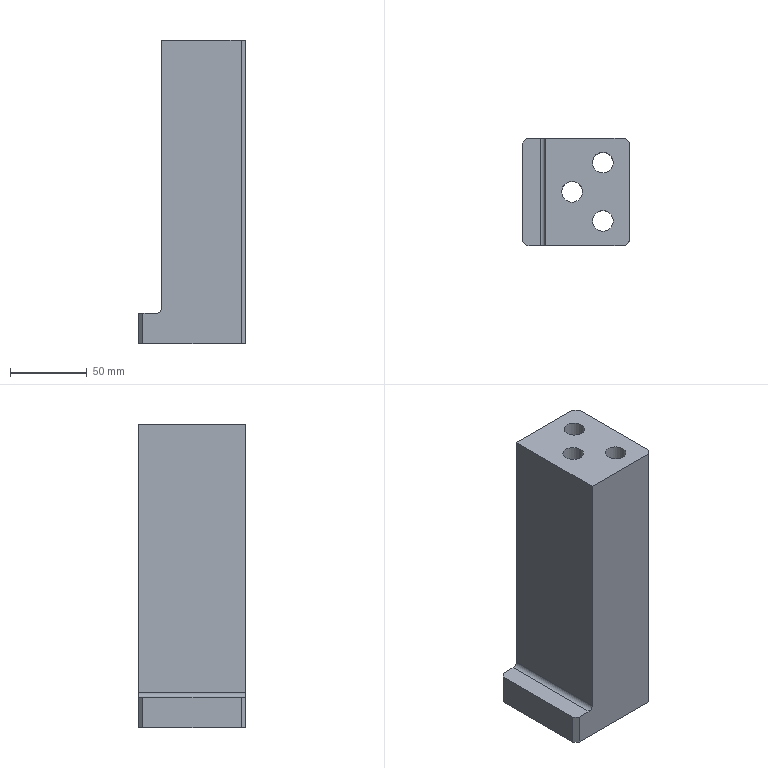Part | NX | features solid 2 | 1 solid | 22 faces | box 70 x 70 x 198 mm | volume 634687 mm3 | plane 15 | cylinder 7 | commonest cylinder face diameters 13.507 x3 20.008 x3 6 x1
STEP:
#1=CARTESIAN_POINT('',(964.467,186.199,-16.87));
#2=VERTEX_POINT('',#1);
#3=CARTESIAN_POINT('',(964.467,122.199,-16.87));
#4=VERTEX_POINT('',#3);
#5=CARTESIAN_POINT('',(964.467,12.095,-16.87));
#6=DIRECTION('',(0.,-1.,0.));
#7=VECTOR('',#6,1000.);
#8=LINE('',#5,#7);
#9=EDGE_CURVE('',#2,#4,#8,.T.);
#10=ORIENTED_EDGE('',*,*,#9,.T.);
#11=CARTESIAN_POINT('',(961.467,119.199,-16.87));
#12=VERTEX_POINT('',#11);
#13=CARTESIAN_POINT('',(777.169,-65.098,-16.87));
#14=DIRECTION('',(0.7071,0.7071,0.));
#15=VECTOR('',#14,1000.);
#16=LINE('',#13,#15);
#17=EDGE_CURVE('',#4,#12,#16,.F.);
#18=ORIENTED_EDGE('',*,*,#17,.T.);
#19=CARTESIAN_POINT('',(897.467,119.199,-16.87));
#20=VERTEX_POINT('',#19);
#21=CARTESIAN_POINT('',(699.976,119.199,-16.87));
#22=DIRECTION('',(-1.,0.,0.));
#23=VECTOR('',#22,1000.);
#24=LINE('',#21,#23);
#25=EDGE_CURVE('',#12,#20,#24,.T.);
#26=ORIENTED_EDGE('',*,*,#25,.T.);
#27=CARTESIAN_POINT('',(894.467,122.199,-16.87));
#28=VERTEX_POINT('',#27);
#29=CARTESIAN_POINT('',(852.274,164.392,-16.87));
#30=DIRECTION('',(0.7071,-0.7071,0.));
#31=VECTOR('',#30,1000.);
#32=LINE('',#29,#31);
#33=EDGE_CURVE('',#20,#28,#32,.F.);
#34=ORIENTED_EDGE('',*,*,#33,.T.);
#35=CARTESIAN_POINT('',(894.467,186.199,-16.87));
#36=VERTEX_POINT('',#35);
#37=CARTESIAN_POINT('',(894.467,12.095,-16.87));
#38=DIRECTION('',(0.,1.,0.));
#39=VECTOR('',#38,1000.);
#40=LINE('',#37,#39);
#41=EDGE_CURVE('',#28,#36,#40,.T.);
#42=ORIENTED_EDGE('',*,*,#41,.T.);
#43=CARTESIAN_POINT('',(897.467,189.199,-16.87));
#44=VERTEX_POINT('',#43);
#45=CARTESIAN_POINT('',(710.169,1.902,-16.87));
#46=DIRECTION('',(-0.7071,-0.7071,0.));
#47=VECTOR('',#46,1000.);
#48=LINE('',#45,#47);
#49=EDGE_CURVE('',#36,#44,#48,.F.);
#50=ORIENTED_EDGE('',*,*,#49,.T.);
#51=CARTESIAN_POINT('',(961.467,189.199,-16.87));
#52=VERTEX_POINT('',#51);
#53=CARTESIAN_POINT('',(699.976,189.199,-16.87));
#54=DIRECTION('',(1.,0.,0.));
#55=VECTOR('',#54,1000.);
#56=LINE('',#53,#55);
#57=EDGE_CURVE('',#44,#52,#56,.T.);
#58=ORIENTED_EDGE('',*,*,#57,.T.);
#59=CARTESIAN_POINT('',(919.274,231.392,-16.87));
#60=DIRECTION('',(-0.7071,0.7071,0.));
#61=VECTOR('',#60,1000.);
#62=LINE('',#59,#61);
#63=EDGE_CURVE('',#52,#2,#62,.F.);
#64=ORIENTED_EDGE('',*,*,#63,.T.);
#65=EDGE_LOOP('',(#10,#18,#26,#34,#42,#50,#58,#64));
#66=FACE_BOUND('',#65,.T.);
#67=CARTESIAN_POINT('',(936.963,135.199,-16.87));
#68=VERTEX_POINT('',#67);
#69=CARTESIAN_POINT('',(946.967,135.199,-16.87));
#70=DIRECTION('',(0.,0.,-1.));
#71=DIRECTION('',(-1.,0.,0.));
#72=AXIS2_PLACEMENT_3D('',#69,#70,#71);
#73=CIRCLE('',#72,10.004);
#74=EDGE_CURVE('',#68,#68,#73,.T.);
#75=ORIENTED_EDGE('',*,*,#74,.F.);
#76=EDGE_LOOP('',(#75));
#77=FACE_BOUND('',#76,.T.);
#78=CARTESIAN_POINT('',(936.963,173.199,-16.87));
#79=VERTEX_POINT('',#78);
#80=CARTESIAN_POINT('',(946.967,173.199,-16.87));
#81=DIRECTION('',(0.,0.,-1.));
#82=DIRECTION('',(-1.,0.,0.));
#83=AXIS2_PLACEMENT_3D('',#80,#81,#82);
#84=CIRCLE('',#83,10.004);
#85=EDGE_CURVE('',#79,#79,#84,.T.);
#86=ORIENTED_EDGE('',*,*,#85,.F.);
#87=EDGE_LOOP('',(#86));
#88=FACE_BOUND('',#87,.T.);
#89=CARTESIAN_POINT('',(916.963,154.199,-16.87));
#90=VERTEX_POINT('',#89);
#91=CARTESIAN_POINT('',(926.967,154.199,-16.87));
#92=DIRECTION('',(0.,0.,-1.));
#93=DIRECTION('',(-1.,0.,0.));
#94=AXIS2_PLACEMENT_3D('',#91,#92,#93);
#95=CIRCLE('',#94,10.004);
#96=EDGE_CURVE('',#90,#90,#95,.F.);
#97=ORIENTED_EDGE('',*,*,#96,.T.);
#98=EDGE_LOOP('',(#97));
#99=FACE_BOUND('',#98,.T.);
#100=CARTESIAN_POINT('',(699.976,12.095,-16.87));
#101=DIRECTION('',(0.,0.,-1.));
#102=DIRECTION('',(-1.,0.,0.));
#103=AXIS2_PLACEMENT_3D('',#100,#101,#102);
#104=PLANE('',#103);
#105=ADVANCED_FACE('',(#66,#77,#88,#99),#104,.T.);
#106=CARTESIAN_POINT('',(894.467,186.199,2.999));
#107=VERTEX_POINT('',#106);
#108=CARTESIAN_POINT('',(894.467,122.199,2.999));
#109=VERTEX_POINT('',#108);
#110=CARTESIAN_POINT('',(894.467,189.199,2.999));
#111=DIRECTION('',(0.,1.,0.));
#112=VECTOR('',#111,1000.);
#113=LINE('',#110,#112);
#114=EDGE_CURVE('',#107,#109,#113,.F.);
#115=ORIENTED_EDGE('',*,*,#114,.T.);
#116=CARTESIAN_POINT('',(897.467,119.199,2.999));
#117=VERTEX_POINT('',#116);
#118=CARTESIAN_POINT('',(894.467,122.199,2.999));
#119=DIRECTION('',(0.7071,-0.7071,0.));
#120=VECTOR('',#119,1000.);
#121=LINE('',#118,#120);
#122=EDGE_CURVE('',#109,#117,#121,.T.);
#123=ORIENTED_EDGE('',*,*,#122,.T.);
#124=CARTESIAN_POINT('',(906.467,119.199,2.999));
#125=VERTEX_POINT('',#124);
#126=CARTESIAN_POINT('',(894.467,119.199,2.999));
#127=DIRECTION('',(-1.,0.,0.));
#128=VECTOR('',#127,1000.);
#129=LINE('',#126,#128);
#130=EDGE_CURVE('',#117,#125,#129,.F.);
#131=ORIENTED_EDGE('',*,*,#130,.T.);
#132=CARTESIAN_POINT('',(906.467,189.199,2.999));
#133=VERTEX_POINT('',#132);
#134=CARTESIAN_POINT('',(906.467,154.199,2.999));
#135=DIRECTION('',(0.,1.,0.));
#136=VECTOR('',#135,1000.);
#137=LINE('',#134,#136);
#138=EDGE_CURVE('',#125,#133,#137,.T.);
#139=ORIENTED_EDGE('',*,*,#138,.T.);
#140=CARTESIAN_POINT('',(897.467,189.199,2.999));
#141=VERTEX_POINT('',#140);
#142=CARTESIAN_POINT('',(959.467,189.199,2.999));
#143=DIRECTION('',(1.,0.,0.));
#144=VECTOR('',#143,1000.);
#145=LINE('',#142,#144);
#146=EDGE_CURVE('',#133,#141,#145,.F.);
#147=ORIENTED_EDGE('',*,*,#146,.T.);
#148=CARTESIAN_POINT('',(897.467,189.199,2.999));
#149=DIRECTION('',(-0.7071,-0.7071,0.));
#150=VECTOR('',#149,1000.);
#151=LINE('',#148,#150);
#152=EDGE_CURVE('',#141,#107,#151,.T.);
#153=ORIENTED_EDGE('',*,*,#152,.T.);
#154=EDGE_LOOP('',(#115,#123,#131,#139,#147,#153));
#155=FACE_BOUND('',#154,.T.);
#156=CARTESIAN_POINT('',(926.967,154.199,2.999));
#157=DIRECTION('',(0.,0.,-1.));
#158=DIRECTION('',(0.,-1.,0.));
#159=AXIS2_PLACEMENT_3D('',#156,#157,#158);
#160=PLANE('',#159);
#161=ADVANCED_FACE('',(#155),#160,.F.);
#162=CARTESIAN_POINT('',(909.467,119.199,5.999));
#163=VERTEX_POINT('',#162);
#164=CARTESIAN_POINT('',(906.467,119.199,5.999));
#165=DIRECTION('',(0.,1.,0.));
#166=DIRECTION('',(0.,0.,1.));
#167=AXIS2_PLACEMENT_3D('',#164,#165,#166);
#168=CIRCLE('',#167,3.);
#169=EDGE_CURVE('',#163,#125,#168,.T.);
#170=ORIENTED_EDGE('',*,*,#169,.F.);
#171=CARTESIAN_POINT('',(909.467,189.199,5.999));
#172=VERTEX_POINT('',#171);
#173=CARTESIAN_POINT('',(909.467,189.199,5.999));
#174=DIRECTION('',(0.,1.,0.));
#175=VECTOR('',#174,1000.);
#176=LINE('',#173,#175);
#177=EDGE_CURVE('',#172,#163,#176,.F.);
#178=ORIENTED_EDGE('',*,*,#177,.F.);
#179=CARTESIAN_POINT('',(906.467,189.199,5.999));
#180=DIRECTION('',(0.,-1.,0.));
#181=DIRECTION('',(0.,0.,-1.));
#182=AXIS2_PLACEMENT_3D('',#179,#180,#181);
#183=CIRCLE('',#182,3.);
#184=EDGE_CURVE('',#133,#172,#183,.T.);
#185=ORIENTED_EDGE('',*,*,#184,.F.);
#186=ORIENTED_EDGE('',*,*,#138,.F.);
#187=EDGE_LOOP('',(#170,#178,#185,#186));
#188=FACE_BOUND('',#187,.T.);
#189=CARTESIAN_POINT('',(906.467,189.199,5.999));
#190=DIRECTION('',(0.,1.,0.));
#191=DIRECTION('',(0.,0.,-1.));
#192=AXIS2_PLACEMENT_3D('',#189,#190,#191);
#193=CYLINDRICAL_SURFACE('',#192,3.);
#194=ADVANCED_FACE('',(#188),#193,.F.);
#195=CARTESIAN_POINT('',(909.467,119.199,181.13));
#196=VERTEX_POINT('',#195);
#197=CARTESIAN_POINT('',(909.467,119.199,194.799));
#198=DIRECTION('',(0.,0.,-1.));
#199=VECTOR('',#198,1000.);
#200=LINE('',#197,#199);
#201=EDGE_CURVE('',#163,#196,#200,.F.);
#202=ORIENTED_EDGE('',*,*,#201,.T.);
#203=CARTESIAN_POINT('',(909.467,189.199,181.13));
#204=VERTEX_POINT('',#203);
#205=CARTESIAN_POINT('',(909.467,-371.311,181.13));
#206=DIRECTION('',(0.,1.,0.));
#207=VECTOR('',#206,1000.);
#208=LINE('',#205,#207);
#209=EDGE_CURVE('',#196,#204,#208,.T.);
#210=ORIENTED_EDGE('',*,*,#209,.T.);
#211=CARTESIAN_POINT('',(909.467,189.199,194.799));
#212=DIRECTION('',(0.,0.,-1.));
#213=VECTOR('',#212,1000.);
#214=LINE('',#211,#213);
#215=EDGE_CURVE('',#172,#204,#214,.F.);
#216=ORIENTED_EDGE('',*,*,#215,.F.);
#217=ORIENTED_EDGE('',*,*,#177,.T.);
#218=EDGE_LOOP('',(#202,#210,#216,#217));
#219=FACE_BOUND('',#218,.T.);
#220=CARTESIAN_POINT('',(909.467,189.199,194.799));
#221=DIRECTION('',(-1.,0.,0.));
#222=DIRECTION('',(0.,0.,-1.));
#223=AXIS2_PLACEMENT_3D('',#220,#221,#222);
#224=PLANE('',#223);
#225=ADVANCED_FACE('',(#219),#224,.T.);
#226=CARTESIAN_POINT('',(961.467,119.199,181.13));
#227=VERTEX_POINT('',#226);
#228=CARTESIAN_POINT('',(964.467,122.199,181.13));
#229=VERTEX_POINT('',#228);
#230=CARTESIAN_POINT('',(961.467,119.199,181.13));
#231=DIRECTION('',(-0.7071,-0.7071,0.));
#232=VECTOR('',#231,1000.);
#233=LINE('',#230,#232);
#234=EDGE_CURVE('',#227,#229,#233,.F.);
#235=ORIENTED_EDGE('',*,*,#234,.F.);
#236=CARTESIAN_POINT('',(961.467,119.199,194.799));
#237=DIRECTION('',(0.,0.,-1.));
#238=VECTOR('',#237,1000.);
#239=LINE('',#236,#238);
#240=EDGE_CURVE('',#12,#227,#239,.F.);
#241=ORIENTED_EDGE('',*,*,#240,.F.);
#242=ORIENTED_EDGE('',*,*,#17,.F.);
#243=CARTESIAN_POINT('',(964.467,122.199,194.799));
#244=DIRECTION('',(0.,0.,1.));
#245=VECTOR('',#244,1000.);
#246=LINE('',#243,#245);
#247=EDGE_CURVE('',#229,#4,#246,.F.);
#248=ORIENTED_EDGE('',*,*,#247,.F.);
#249=EDGE_LOOP('',(#235,#241,#242,#248));
#250=FACE_BOUND('',#249,.T.);
#251=CARTESIAN_POINT('',(961.467,119.199,194.799));
#252=DIRECTION('',(-0.7071,0.7071,0.));
#253=DIRECTION('',(0.7071,0.7071,0.));
#254=AXIS2_PLACEMENT_3D('',#251,#252,#253);
#255=PLANE('',#254);
#256=ADVANCED_FACE('',(#250),#255,.F.);
#257=CARTESIAN_POINT('',(729.857,119.199,181.13));
#258=DIRECTION('',(-1.,0.,0.));
#259=VECTOR('',#258,1000.);
#260=LINE('',#257,#259);
#261=EDGE_CURVE('',#227,#196,#260,.T.);
#262=ORIENTED_EDGE('',*,*,#261,.T.);
#263=ORIENTED_EDGE('',*,*,#201,.F.);
#264=ORIENTED_EDGE('',*,*,#169,.T.);
#265=ORIENTED_EDGE('',*,*,#130,.F.);
#266=CARTESIAN_POINT('',(897.467,119.199,122.999));
#267=DIRECTION('',(0.,0.,1.));
#268=VECTOR('',#267,1000.);
#269=LINE('',#266,#268);
#270=EDGE_CURVE('',#117,#20,#269,.F.);
#271=ORIENTED_EDGE('',*,*,#270,.T.);
#272=ORIENTED_EDGE('',*,*,#25,.F.);
#273=ORIENTED_EDGE('',*,*,#240,.T.);
#274=EDGE_LOOP('',(#262,#263,#264,#265,#271,#272,#273));
#275=FACE_BOUND('',#274,.T.);
#276=CARTESIAN_POINT('',(894.467,119.199,194.799));
#277=DIRECTION('',(0.,-1.,0.));
#278=DIRECTION('',(0.,0.,1.));
#279=AXIS2_PLACEMENT_3D('',#276,#277,#278);
#280=PLANE('',#279);
#281=ADVANCED_FACE('',(#275),#280,.T.);
#282=ORIENTED_EDGE('',*,*,#122,.F.);
#283=CARTESIAN_POINT('',(894.467,122.199,122.999));
#284=DIRECTION('',(0.,0.,-1.));
#285=VECTOR('',#284,1000.);
#286=LINE('',#283,#285);
#287=EDGE_CURVE('',#28,#109,#286,.F.);
#288=ORIENTED_EDGE('',*,*,#287,.F.);
#289=ORIENTED_EDGE('',*,*,#33,.F.);
#290=ORIENTED_EDGE('',*,*,#270,.F.);
#291=EDGE_LOOP('',(#282,#288,#289,#290));
#292=FACE_BOUND('',#291,.T.);
#293=CARTESIAN_POINT('',(894.467,122.199,122.999));
#294=DIRECTION('',(0.7071,0.7071,0.));
#295=DIRECTION('',(0.7071,-0.7071,0.));
#296=AXIS2_PLACEMENT_3D('',#293,#294,#295);
#297=PLANE('',#296);
#298=ADVANCED_FACE('',(#292),#297,.F.);
#299=ORIENTED_EDGE('',*,*,#41,.F.);
#300=ORIENTED_EDGE('',*,*,#287,.T.);
#301=ORIENTED_EDGE('',*,*,#114,.F.);
#302=CARTESIAN_POINT('',(894.467,186.199,122.999));
#303=DIRECTION('',(0.,0.,1.));
#304=VECTOR('',#303,1000.);
#305=LINE('',#302,#304);
#306=EDGE_CURVE('',#107,#36,#305,.F.);
#307=ORIENTED_EDGE('',*,*,#306,.T.);
#308=EDGE_LOOP('',(#299,#300,#301,#307));
#309=FACE_BOUND('',#308,.T.);
#310=CARTESIAN_POINT('',(894.467,189.199,122.999));
#311=DIRECTION('',(-1.,0.,0.));
#312=DIRECTION('',(0.,0.,-1.));
#313=AXIS2_PLACEMENT_3D('',#310,#311,#312);
#314=PLANE('',#313);
#315=ADVANCED_FACE('',(#309),#314,.T.);
#316=ORIENTED_EDGE('',*,*,#152,.F.);
#317=CARTESIAN_POINT('',(897.467,189.199,122.999));
#318=DIRECTION('',(0.,0.,-1.));
#319=VECTOR('',#318,1000.);
#320=LINE('',#317,#319);
#321=EDGE_CURVE('',#44,#141,#320,.F.);
#322=ORIENTED_EDGE('',*,*,#321,.F.);
#323=ORIENTED_EDGE('',*,*,#49,.F.);
#324=ORIENTED_EDGE('',*,*,#306,.F.);
#325=EDGE_LOOP('',(#316,#322,#323,#324));
#326=FACE_BOUND('',#325,.T.);
#327=CARTESIAN_POINT('',(897.467,189.199,122.999));
#328=DIRECTION('',(0.7071,-0.7071,0.));
#329=DIRECTION('',(-0.7071,-0.7071,0.));
#330=AXIS2_PLACEMENT_3D('',#327,#328,#329);
#331=PLANE('',#330);
#332=ADVANCED_FACE('',(#326),#331,.F.);
#333=ORIENTED_EDGE('',*,*,#57,.F.);
#334=ORIENTED_EDGE('',*,*,#321,.T.);
#335=ORIENTED_EDGE('',*,*,#146,.F.);
#336=ORIENTED_EDGE('',*,*,#184,.T.);
#337=ORIENTED_EDGE('',*,*,#215,.T.);
#338=CARTESIAN_POINT('',(961.467,189.199,181.13));
#339=VERTEX_POINT('',#338);
#340=CARTESIAN_POINT('',(729.857,189.199,181.13));
#341=DIRECTION('',(1.,0.,0.));
#342=VECTOR('',#341,1000.);
#343=LINE('',#340,#342);
#344=EDGE_CURVE('',#204,#339,#343,.T.);
#345=ORIENTED_EDGE('',*,*,#344,.T.);
#346=CARTESIAN_POINT('',(961.467,189.199,194.799));
#347=DIRECTION('',(0.,0.,1.));
#348=VECTOR('',#347,1000.);
#349=LINE('',#346,#348);
#350=EDGE_CURVE('',#339,#52,#349,.F.);
#351=ORIENTED_EDGE('',*,*,#350,.T.);
#352=EDGE_LOOP('',(#333,#334,#335,#336,#337,#345,#351));
#353=FACE_BOUND('',#352,.T.);
#354=CARTESIAN_POINT('',(959.467,189.199,194.799));
#355=DIRECTION('',(0.,1.,0.));
#356=DIRECTION('',(0.,0.,-1.));
#357=AXIS2_PLACEMENT_3D('',#354,#355,#356);
#358=PLANE('',#357);
#359=ADVANCED_FACE('',(#353),#358,.T.);
#360=CARTESIAN_POINT('',(964.467,186.199,181.13));
#361=VERTEX_POINT('',#360);
#362=CARTESIAN_POINT('',(964.467,186.199,181.13));
#363=DIRECTION('',(0.7071,-0.7071,0.));
#364=VECTOR('',#363,1000.);
#365=LINE('',#362,#364);
#366=EDGE_CURVE('',#361,#339,#365,.F.);
#367=ORIENTED_EDGE('',*,*,#366,.F.);
#368=CARTESIAN_POINT('',(964.467,186.199,194.799));
#369=DIRECTION('',(0.,0.,-1.));
#370=VECTOR('',#369,1000.);
#371=LINE('',#368,#370);
#372=EDGE_CURVE('',#2,#361,#371,.F.);
#373=ORIENTED_EDGE('',*,*,#372,.F.);
#374=ORIENTED_EDGE('',*,*,#63,.F.);
#375=ORIENTED_EDGE('',*,*,#350,.F.);
#376=EDGE_LOOP('',(#367,#373,#374,#375));
#377=FACE_BOUND('',#376,.T.);
#378=CARTESIAN_POINT('',(964.467,186.199,194.799));
#379=DIRECTION('',(-0.7071,-0.7071,0.));
#380=DIRECTION('',(-0.7071,0.7071,0.));
#381=AXIS2_PLACEMENT_3D('',#378,#379,#380);
#382=PLANE('',#381);
#383=ADVANCED_FACE('',(#377),#382,.F.);
#384=CARTESIAN_POINT('',(964.467,-371.311,181.13));
#385=DIRECTION('',(0.,-1.,0.));
#386=VECTOR('',#385,1000.);
#387=LINE('',#384,#386);
#388=EDGE_CURVE('',#361,#229,#387,.T.);
#389=ORIENTED_EDGE('',*,*,#388,.T.);
#390=ORIENTED_EDGE('',*,*,#247,.T.);
#391=ORIENTED_EDGE('',*,*,#9,.F.);
#392=ORIENTED_EDGE('',*,*,#372,.T.);
#393=EDGE_LOOP('',(#389,#390,#391,#392));
#394=FACE_BOUND('',#393,.T.);
#395=CARTESIAN_POINT('',(964.467,119.199,194.799));
#396=DIRECTION('',(1.,0.,0.));
#397=DIRECTION('',(0.,0.,1.));
#398=AXIS2_PLACEMENT_3D('',#395,#396,#397);
#399=PLANE('',#398);
#400=ADVANCED_FACE('',(#394),#399,.T.);
#401=CARTESIAN_POINT('',(920.213,154.199,181.13));
#402=VERTEX_POINT('',#401);
#403=CARTESIAN_POINT('',(926.967,154.199,181.13));
#404=DIRECTION('',(0.,0.,-1.));
#405=DIRECTION('',(-1.,0.,0.));
#406=AXIS2_PLACEMENT_3D('',#403,#404,#405);
#407=CIRCLE('',#406,6.753);
#408=EDGE_CURVE('',#402,#402,#407,.T.);
#409=ORIENTED_EDGE('',*,*,#408,.T.);
#410=EDGE_LOOP('',(#409));
#411=FACE_BOUND('',#410,.T.);
#412=CARTESIAN_POINT('',(946.967,166.446,181.13));
#413=VERTEX_POINT('',#412);
#414=CARTESIAN_POINT('',(946.967,173.199,181.13));
#415=DIRECTION('',(0.,0.,-1.));
#416=DIRECTION('',(0.,-1.,0.));
#417=AXIS2_PLACEMENT_3D('',#414,#415,#416);
#418=CIRCLE('',#417,6.753);
#419=EDGE_CURVE('',#413,#413,#418,.T.);
#420=ORIENTED_EDGE('',*,*,#419,.T.);
#421=EDGE_LOOP('',(#420));
#422=FACE_BOUND('',#421,.T.);
#423=CARTESIAN_POINT('',(946.967,128.446,181.13));
#424=VERTEX_POINT('',#423);
#425=CARTESIAN_POINT('',(946.967,135.199,181.13));
#426=DIRECTION('',(0.,0.,-1.));
#427=DIRECTION('',(0.,-1.,0.));
#428=AXIS2_PLACEMENT_3D('',#425,#426,#427);
#429=CIRCLE('',#428,6.753);
#430=EDGE_CURVE('',#424,#424,#429,.T.);
#431=ORIENTED_EDGE('',*,*,#430,.T.);
#432=EDGE_LOOP('',(#431));
#433=FACE_BOUND('',#432,.T.);
#434=ORIENTED_EDGE('',*,*,#344,.F.);
#435=ORIENTED_EDGE('',*,*,#209,.F.);
#436=ORIENTED_EDGE('',*,*,#261,.F.);
#437=ORIENTED_EDGE('',*,*,#234,.T.);
#438=ORIENTED_EDGE('',*,*,#388,.F.);
#439=ORIENTED_EDGE('',*,*,#366,.T.);
#440=EDGE_LOOP('',(#434,#435,#436,#437,#438,#439));
#441=FACE_BOUND('',#440,.T.);
#442=CARTESIAN_POINT('',(729.857,-371.311,181.13));
#443=DIRECTION('',(0.,0.,-1.));
#444=DIRECTION('',(-1.,0.,0.));
#445=AXIS2_PLACEMENT_3D('',#442,#443,#444);
#446=PLANE('',#445);
#447=ADVANCED_FACE('',(#411,#422,#433,#441),#446,.F.);
#448=CARTESIAN_POINT('',(946.967,128.446,102.999));
#449=VERTEX_POINT('',#448);
#450=CARTESIAN_POINT('',(946.967,135.199,102.999));
#451=DIRECTION('',(0.,0.,-1.));
#452=DIRECTION('',(0.,-1.,0.));
#453=AXIS2_PLACEMENT_3D('',#450,#451,#452);
#454=CIRCLE('',#453,6.753);
#455=EDGE_CURVE('',#449,#449,#454,.T.);
#456=ORIENTED_EDGE('',*,*,#455,.T.);
#457=EDGE_LOOP('',(#456));
#458=FACE_BOUND('',#457,.T.);
#459=ORIENTED_EDGE('',*,*,#430,.F.);
#460=EDGE_LOOP('',(#459));
#461=FACE_BOUND('',#460,.T.);
#462=CARTESIAN_POINT('',(946.967,135.199,198.999));
#463=DIRECTION('',(0.,0.,-1.));
#464=DIRECTION('',(0.,-1.,0.));
#465=AXIS2_PLACEMENT_3D('',#462,#463,#464);
#466=CYLINDRICAL_SURFACE('',#465,6.753);
#467=ADVANCED_FACE('',(#458,#461),#466,.F.);
#468=ORIENTED_EDGE('',*,*,#74,.T.);
#469=EDGE_LOOP('',(#468));
#470=FACE_BOUND('',#469,.T.);
#471=CARTESIAN_POINT('',(946.967,125.195,102.999));
#472=VERTEX_POINT('',#471);
#473=CARTESIAN_POINT('',(946.967,135.199,102.999));
#474=DIRECTION('',(0.,0.,-1.));
#475=DIRECTION('',(0.,-1.,0.));
#476=AXIS2_PLACEMENT_3D('',#473,#474,#475);
#477=CIRCLE('',#476,10.004);
#478=EDGE_CURVE('',#472,#472,#477,.F.);
#479=ORIENTED_EDGE('',*,*,#478,.T.);
#480=EDGE_LOOP('',(#479));
#481=FACE_BOUND('',#480,.T.);
#482=CARTESIAN_POINT('',(946.967,135.199,132.999));
#483=DIRECTION('',(0.,0.,-1.));
#484=DIRECTION('',(0.,-1.,0.));
#485=AXIS2_PLACEMENT_3D('',#482,#483,#484);
#486=CYLINDRICAL_SURFACE('',#485,10.004);
#487=ADVANCED_FACE('',(#470,#481),#486,.F.);
#488=ORIENTED_EDGE('',*,*,#455,.F.);
#489=EDGE_LOOP('',(#488));
#490=FACE_BOUND('',#489,.T.);
#491=ORIENTED_EDGE('',*,*,#478,.F.);
#492=EDGE_LOOP('',(#491));
#493=FACE_BOUND('',#492,.T.);
#494=CARTESIAN_POINT('',(946.967,135.199,102.999));
#495=DIRECTION('',(0.,0.,-1.));
#496=DIRECTION('',(0.,-1.,0.));
#497=AXIS2_PLACEMENT_3D('',#494,#495,#496);
#498=PLANE('',#497);
#499=ADVANCED_FACE('',(#490,#493),#498,.T.);
#500=CARTESIAN_POINT('',(946.967,166.446,102.999));
#501=VERTEX_POINT('',#500);
#502=CARTESIAN_POINT('',(946.967,173.199,102.999));
#503=DIRECTION('',(0.,0.,-1.));
#504=DIRECTION('',(0.,-1.,0.));
#505=AXIS2_PLACEMENT_3D('',#502,#503,#504);
#506=CIRCLE('',#505,6.753);
#507=EDGE_CURVE('',#501,#501,#506,.T.);
#508=ORIENTED_EDGE('',*,*,#507,.T.);
#509=EDGE_LOOP('',(#508));
#510=FACE_BOUND('',#509,.T.);
#511=ORIENTED_EDGE('',*,*,#419,.F.);
#512=EDGE_LOOP('',(#511));
#513=FACE_BOUND('',#512,.T.);
#514=CARTESIAN_POINT('',(946.967,173.199,198.999));
#515=DIRECTION('',(0.,0.,-1.));
#516=DIRECTION('',(0.,-1.,0.));
#517=AXIS2_PLACEMENT_3D('',#514,#515,#516);
#518=CYLINDRICAL_SURFACE('',#517,6.753);
#519=ADVANCED_FACE('',(#510,#513),#518,.F.);
#520=ORIENTED_EDGE('',*,*,#85,.T.);
#521=EDGE_LOOP('',(#520));
#522=FACE_BOUND('',#521,.T.);
#523=CARTESIAN_POINT('',(946.967,163.195,102.999));
#524=VERTEX_POINT('',#523);
#525=CARTESIAN_POINT('',(946.967,173.199,102.999));
#526=DIRECTION('',(0.,0.,-1.));
#527=DIRECTION('',(0.,-1.,0.));
#528=AXIS2_PLACEMENT_3D('',#525,#526,#527);
#529=CIRCLE('',#528,10.004);
#530=EDGE_CURVE('',#524,#524,#529,.F.);
#531=ORIENTED_EDGE('',*,*,#530,.T.);
#532=EDGE_LOOP('',(#531));
#533=FACE_BOUND('',#532,.T.);
#534=CARTESIAN_POINT('',(946.967,173.199,132.999));
#535=DIRECTION('',(0.,0.,-1.));
#536=DIRECTION('',(0.,-1.,0.));
#537=AXIS2_PLACEMENT_3D('',#534,#535,#536);
#538=CYLINDRICAL_SURFACE('',#537,10.004);
#539=ADVANCED_FACE('',(#522,#533),#538,.F.);
#540=ORIENTED_EDGE('',*,*,#507,.F.);
#541=EDGE_LOOP('',(#540));
#542=FACE_BOUND('',#541,.T.);
#543=ORIENTED_EDGE('',*,*,#530,.F.);
#544=EDGE_LOOP('',(#543));
#545=FACE_BOUND('',#544,.T.);
#546=CARTESIAN_POINT('',(946.967,173.199,102.999));
#547=DIRECTION('',(0.,0.,-1.));
#548=DIRECTION('',(0.,-1.,0.));
#549=AXIS2_PLACEMENT_3D('',#546,#547,#548);
#550=PLANE('',#549);
#551=ADVANCED_FACE('',(#542,#545),#550,.T.);
#552=CARTESIAN_POINT('',(920.213,154.199,102.999));
#553=VERTEX_POINT('',#552);
#554=CARTESIAN_POINT('',(926.967,154.199,102.999));
#555=DIRECTION('',(0.,0.,1.));
#556=DIRECTION('',(-1.,0.,0.));
#557=AXIS2_PLACEMENT_3D('',#554,#555,#556);
#558=CIRCLE('',#557,6.753);
#559=EDGE_CURVE('',#553,#553,#558,.F.);
#560=ORIENTED_EDGE('',*,*,#559,.F.);
#561=EDGE_LOOP('',(#560));
#562=FACE_BOUND('',#561,.T.);
#563=CARTESIAN_POINT('',(916.963,154.199,102.999));
#564=VERTEX_POINT('',#563);
#565=CARTESIAN_POINT('',(926.967,154.199,102.999));
#566=DIRECTION('',(0.,0.,-1.));
#567=DIRECTION('',(-1.,0.,0.));
#568=AXIS2_PLACEMENT_3D('',#565,#566,#567);
#569=CIRCLE('',#568,10.004);
#570=EDGE_CURVE('',#564,#564,#569,.F.);
#571=ORIENTED_EDGE('',*,*,#570,.F.);
#572=EDGE_LOOP('',(#571));
#573=FACE_BOUND('',#572,.T.);
#574=CARTESIAN_POINT('',(926.967,154.199,102.999));
#575=DIRECTION('',(0.,0.,1.));
#576=DIRECTION('',(0.,1.,0.));
#577=AXIS2_PLACEMENT_3D('',#574,#575,#576);
#578=PLANE('',#577);
#579=ADVANCED_FACE('',(#562,#573),#578,.F.);
#580=ORIENTED_EDGE('',*,*,#96,.F.);
#581=EDGE_LOOP('',(#580));
#582=FACE_BOUND('',#581,.T.);
#583=ORIENTED_EDGE('',*,*,#570,.T.);
#584=EDGE_LOOP('',(#583));
#585=FACE_BOUND('',#584,.T.);
#586=CARTESIAN_POINT('',(926.967,154.199,102.999));
#587=DIRECTION('',(0.,0.,-1.));
#588=DIRECTION('',(-1.,0.,0.));
#589=AXIS2_PLACEMENT_3D('',#586,#587,#588);
#590=CYLINDRICAL_SURFACE('',#589,10.004);
#591=ADVANCED_FACE('',(#582,#585),#590,.F.);
#592=ORIENTED_EDGE('',*,*,#559,.T.);
#593=EDGE_LOOP('',(#592));
#594=FACE_BOUND('',#593,.T.);
#595=ORIENTED_EDGE('',*,*,#408,.F.);
#596=EDGE_LOOP('',(#595));
#597=FACE_BOUND('',#596,.T.);
#598=CARTESIAN_POINT('',(926.967,154.199,181.13));
#599=DIRECTION('',(0.,0.,-1.));
#600=DIRECTION('',(-1.,0.,0.));
#601=AXIS2_PLACEMENT_3D('',#598,#599,#600);
#602=CYLINDRICAL_SURFACE('',#601,6.753);
#603=ADVANCED_FACE('',(#594,#597),#602,.F.);
#604=CLOSED_SHELL('',(#105,#161,#194,#225,#256,#281,#298,#315,#332,#359,#383,#400,#447,#467,#487,#499,#519,#539,#551,#579,#591,#603));
#605=MANIFOLD_SOLID_BREP('',#604);
#606=(LENGTH_UNIT()NAMED_UNIT(*)SI_UNIT(.MILLI.,.METRE.));
#607=UNCERTAINTY_MEASURE_WITH_UNIT(LENGTH_MEASURE(0.00001),#606,'','');
#608=(NAMED_UNIT(*)PLANE_ANGLE_UNIT()SI_UNIT($,.RADIAN.));
#609=(NAMED_UNIT(*)SI_UNIT($,.STERADIAN.)SOLID_ANGLE_UNIT());
#610=(GEOMETRIC_REPRESENTATION_CONTEXT(3)GLOBAL_UNCERTAINTY_ASSIGNED_CONTEXT((#607))GLOBAL_UNIT_ASSIGNED_CONTEXT((#606,#608,#609))REPRESENTATION_CONTEXT('',''));
#611=ADVANCED_BREP_SHAPE_REPRESENTATION('',(#605),#610);